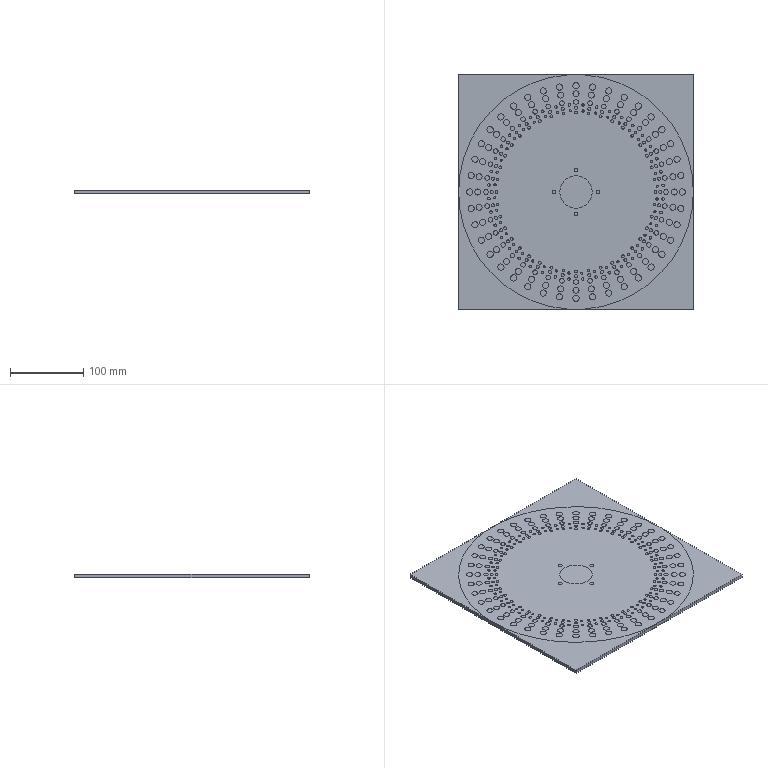NC program | NX | posted with a generic post | part box 320 x 320 x 5 mm
Lines 39370 to 39665 of 63198:
(G81点孔 , TOOL : D6点孔钻)
N78738 T01 M6
N78740 /M1
N78742 G54
N78744 G17 G0 G90 X0. Y-30.1 S1500 M3
N78746 G43 Z20. H1
N78748 G94 G81 G98 Z-1.5 F60. R1.5
N78750 Y0.
N78752 X-30.1
N78754 X0. Y30.1
N78756 X30.1 Y0.
N78758 X103.105 Y33.501
N78760 X102.828 Y41.545
N78762 X110.087 Y45.349
N78764 X102.179 Y52.063
N78766 X96.595 Y49.217
N78768 X95.063 Y57.119
N78770 X101.637 Y62.012
N78772 X109.283 Y55.682
N78774 X119.17 Y60.72
N78776 X128.97 Y65.714
N78778 X117.103 Y85.08
N78780 X108.204 Y78.615
N78782 X99.226 Y72.092
N78784 X92.777 Y67.406
N78786 X87.706 Y63.722
N78788 X84.957 Y71.287
N78790 X90.685 Y77.148
N78792 X81.09 Y81.09
N78794 X76.658 Y76.658
N78796 X72.759 Y83.699
N78798 X77.5 Y90.384
N78800 X86.727 Y86.727
N78802 X94.574 Y94.574
N78804 X102.351 Y102.351
N78806 X85.08 Y117.103
N78808 X78.615 Y108.204
N78810 X72.092 Y99.226
N78812 X67.406 Y92.777
N78814 X63.722 Y87.706
N78816 X58.77 Y94.051
N78818 X49.217 Y96.595
N78820 X43.334 Y102.087
N78822 X45.777 Y109.909
N78824 X52.063 Y102.179
N78826 X62.407 Y101.395
N78828 X55.682 Y109.283
N78830 X60.72 Y119.17
N78832 X65.714 Y128.97
N78834 X44.729 Y137.662
N78836 X41.33 Y127.201
N78838 X37.901 Y116.648
N78840 X35.438 Y109.066
N78842 X33.501 Y103.105
N78844 X26.83 Y107.609
N78846 X28.019 Y115.717
N78848 X16.959 Y107.076
N78850 X17.94 Y113.267
N78852 X19.187 Y121.141
N78854 X20.923 Y132.101
N78856 X22.643 Y142.965
N78858 X0. Y144.747
N78860 Y133.748
N78862 Y122.651
N78864 X9.572 Y118.676
N78866 X9.666 Y110.481
N78868 X0. Y108.411
N78870 Y114.679
N78872 X-9.111 Y118.712
N78874 X-7.736 Y110.633
N78876 X-16.959 Y107.076
N78878 X-17.94 Y113.267
N78880 X-19.187 Y121.141
N78882 X-20.923 Y132.101
N78884 X-22.643 Y142.965
N78886 X-44.729 Y137.662
N78888 X-41.33 Y127.201
N78890 X-37.901 Y116.648
N78892 X-27.569 Y115.825
N78894 X-24.947 Y108.061
N78896 X-35.438 Y109.066
N78898 X-33.501 Y103.105
N78900 X-41.545 Y102.828
N78902 X-45.349 Y110.087
N78904 X-55.682 Y109.283
N78906 X-60.72 Y119.17
N78908 X-65.714 Y128.97
N78910 X-78.615 Y108.204
N78912 X-85.08 Y117.103
N78914 X-102.351 Y102.351
N78916 X-94.574 Y94.574
N78918 X-86.727 Y86.727
N78920 X-77.148 Y90.685
N78922 X-72.092 Y99.226
N78924 X-62.012 Y101.637
N78926 X-52.063 Y102.179
N78928 X-49.217 Y96.595
N78930 X-57.119 Y95.063
N78932 X-67.406 Y92.777
N78934 X-63.722 Y87.706
N78936 X-71.287 Y84.957
N78938 X-81.09 Y81.09
N78940 X-76.658 Y76.658
N78942 X-83.699 Y72.759
N78944 X-87.706 Y63.722
N78946 X-92.777 Y67.406
N78948 X-90.384 Y77.5
N78950 X-99.226 Y72.092
N78952 X-108.204 Y78.615
N78954 X-117.103 Y85.08
N78956 X-128.97 Y65.714
N78958 X-119.17 Y60.72
N78960 X-127.201 Y41.33
N78962 X-137.662 Y44.729
N78964 X-142.965 Y22.643
N78966 X-132.101 Y20.923
N78968 X-121.141 Y19.187
N78970 X-115.717 Y28.019
N78972 X-116.648 Y37.901
N78974 X-109.909 Y45.777
N78976 X-109.283 Y55.682
N78978 X-101.395 Y62.407
N78980 X-94.051 Y58.77
N78982 X-102.179 Y52.063
N78984 X-96.595 Y49.217
N78986 X-102.087 Y43.334
N78988 X-103.105 Y33.501
N78990 X-109.066 Y35.438
N78992 X-107.609 Y26.83
N78994 X-107.076 Y16.959
N78996 X-113.267 Y17.94
N78998 X-118.676 Y9.572
N79000 X-110.481 Y9.666
N79002 X-108.411 Y0.
N79004 X-110.633 Y-7.736
N79006 X-118.712 Y-9.111
N79008 X-114.679 Y0.
N79010 X-122.651
N79012 X-133.748
N79014 X-144.747
N79016 X-142.965 Y-22.643
N79018 X-132.101 Y-20.923
N79020 X-137.662 Y-44.729
N79022 X-127.201 Y-41.33
N79024 X-116.648 Y-37.901
N79026 X-115.825 Y-27.569
N79028 X-121.141 Y-19.187
N79030 X-113.267 Y-17.94
N79032 X-107.076 Y-16.959
N79034 X-108.061 Y-24.947
N79036 X-109.066 Y-35.438
N79038 X-103.105 Y-33.501
N79040 X-102.828 Y-41.545
N79042 X-96.595 Y-49.217
N79044 X-102.179 Y-52.063
N79046 X-110.087 Y-45.349
N79048 X-128.97 Y-65.714
N79050 X-119.17 Y-60.72
N79052 X-109.283 Y-55.682
N79054 X-101.637 Y-62.012
N79056 X-95.063 Y-57.119
N79058 X-87.706 Y-63.722
N79060 X-84.957 Y-71.287
N79062 X-76.658 Y-76.658
N79064 X-81.09 Y-81.09
N79066 X-86.727 Y-86.727
N79068 X-90.685 Y-77.148
N79070 X-92.777 Y-67.406
N79072 X-99.226 Y-72.092
N79074 X-108.204 Y-78.615
N79076 X-117.103 Y-85.08
N79078 X-102.351 Y-102.351
N79080 X-94.574 Y-94.574
N79082 X-85.08 Y-117.103
N79084 X-78.615 Y-108.204
N79086 X-72.092 Y-99.226
N79088 X-77.5 Y-90.384
N79090 X-72.759 Y-83.699
N79092 X-63.722 Y-87.706
N79094 X-67.406 Y-92.777
N79096 X-62.407 Y-101.395
N79098 X-58.77 Y-94.051
N79100 X-49.217 Y-96.595
N79102 X-43.334 Y-102.087
N79104 X-52.063 Y-102.179
N79106 X-55.682 Y-109.283
N79108 X-60.72 Y-119.17
N79110 X-65.714 Y-128.97
N79112 X-44.729 Y-137.662
N79114 X-41.33 Y-127.201
N79116 X-37.901 Y-116.648
N79118 X-45.777 Y-109.909
N79120 X-35.438 Y-109.066
N79122 X-33.501 Y-103.105
N79124 X-26.83 Y-107.609
N79126 X-28.019 Y-115.717
N79128 X-16.959 Y-107.076
N79130 X-17.94 Y-113.267
N79132 X-19.187 Y-121.141
N79134 X-20.923 Y-132.101
N79136 X-22.643 Y-142.965
N79138 X0. Y-144.747
N79140 Y-133.748
N79142 X22.643 Y-142.965
N79144 X20.923 Y-132.101
N79146 X19.187 Y-121.141
N79148 X9.111 Y-118.712
N79150 X0. Y-122.651
N79152 X-9.572 Y-118.676
N79154 X-9.666 Y-110.481
N79156 X0. Y-114.679
N79158 Y-108.411
N79160 X7.736 Y-110.633
N79162 X17.94 Y-113.267
N79164 X16.959 Y-107.076
N79166 X24.947 Y-108.061
N79168 X27.569 Y-115.825
N79170 X35.438 Y-109.066
N79172 X33.501 Y-103.105
N79174 X41.545 Y-102.828
N79176 X49.217 Y-96.595
N79178 X52.063 Y-102.179
N79180 X45.349 Y-110.087
N79182 X37.901 Y-116.648
N79184 X41.33 Y-127.201
N79186 X44.729 Y-137.662
N79188 X65.714 Y-128.97
N79190 X60.72 Y-119.17
N79192 X55.682 Y-109.283
N79194 X62.012 Y-101.637
N79196 X57.119 Y-95.063
N79198 X67.406 Y-92.777
N79200 X63.722 Y-87.706
N79202 X71.287 Y-84.957
N79204 X77.148 Y-90.685
N79206 X72.092 Y-99.226
N79208 X78.615 Y-108.204
N79210 X85.08 Y-117.103
N79212 X102.351 Y-102.351
N79214 X94.574 Y-94.574
N79216 X86.727 Y-86.727
N79218 X90.384 Y-77.5
N79220 X81.09 Y-81.09
N79222 X76.658 Y-76.658
N79224 X83.699 Y-72.759
N79226 X87.706 Y-63.722
N79228 X92.777 Y-67.406
N79230 X99.226 Y-72.092
N79232 X108.204 Y-78.615
N79234 X117.103 Y-85.08
N79236 X128.97 Y-65.714
N79238 X119.17 Y-60.72
N79240 X109.283 Y-55.682
N79242 X101.395 Y-62.407
N79244 X94.051 Y-58.77
N79246 X102.179 Y-52.063
N79248 X96.595 Y-49.217
N79250 X102.087 Y-43.334
N79252 X109.909 Y-45.777
N79254 X109.066 Y-35.438
N79256 X103.105 Y-33.501
N79258 X107.609 Y-26.83
N79260 X113.267 Y-17.94
N79262 X107.076 Y-16.959
N79264 X110.481 Y-9.666
N79266 X118.676 Y-9.572
N79268 X122.651 Y0.
N79270 X114.679
N79272 X108.411
N79274 X110.633 Y7.736
N79276 X118.712 Y9.111
N79278 X121.141 Y19.187
N79280 X113.267 Y17.94
N79282 X107.076 Y16.959
N79284 X108.061 Y24.947
N79286 X115.825 Y27.569
N79288 X109.066 Y35.438
N79290 X116.648 Y37.901
N79292 X127.201 Y41.33
N79294 X137.662 Y44.729
N79296 X142.965 Y22.643
N79298 X132.101 Y20.923
N79300 X133.748 Y0.
N79302 X144.747
N79304 X142.965 Y-22.643
N79306 X132.101 Y-20.923
N79308 X121.141 Y-19.187
N79310 X115.717 Y-28.019
N79312 X116.648 Y-37.901
N79314 X127.201 Y-41.33
N79316 X137.662 Y-44.729
N79318 G80
N79320 G0 X137.662 Y-44.729 Z20.
N79322 M5